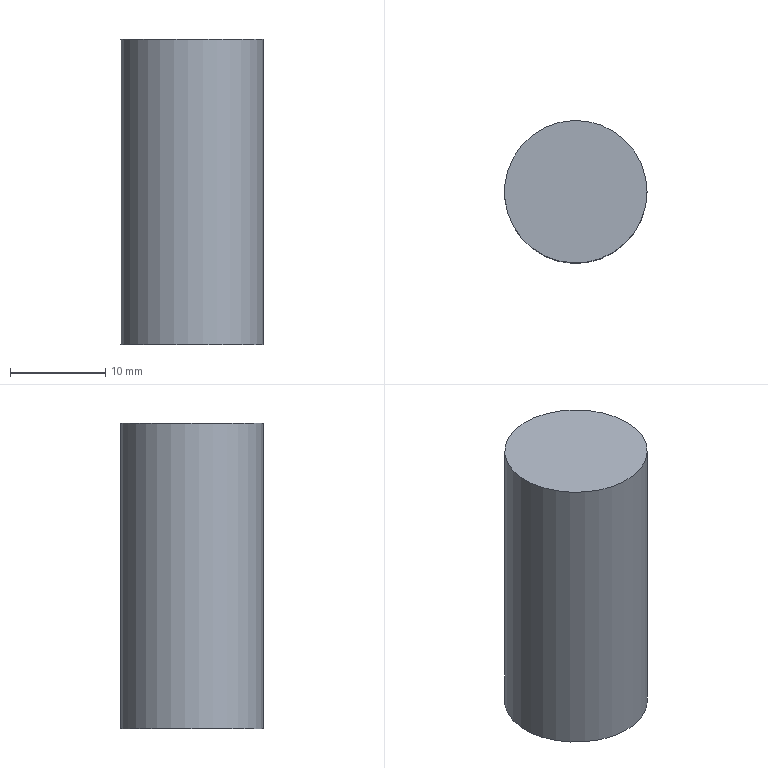Part | NX | features DATUM_CSYS 2, EXTRUDE 1, SKETCH 1 | 1 solid | 3 faces | box 15 x 15 x 32.2 mm | volume 5690 mm3 | plane 2 | cylinder 1 | commonest cylinder face diameters 15 x1
STEP:
#1=CARTESIAN_POINT('',(7.5,0.,32.2));
#2=VERTEX_POINT('',#1);
#3=CARTESIAN_POINT('',(0.,0.,32.2));
#4=DIRECTION('',(0.,0.,1.));
#5=DIRECTION('',(1.,0.,0.));
#6=AXIS2_PLACEMENT_3D('',#3,#4,#5);
#7=CIRCLE('',#6,7.5);
#8=EDGE_CURVE('',#2,#2,#7,.T.);
#9=ORIENTED_EDGE('',*,*,#8,.F.);
#10=EDGE_LOOP('',(#9));
#11=FACE_BOUND('',#10,.T.);
#12=CARTESIAN_POINT('',(7.5,0.,0.));
#13=VERTEX_POINT('',#12);
#14=CARTESIAN_POINT('',(0.,0.,0.));
#15=DIRECTION('',(0.,0.,1.));
#16=DIRECTION('',(1.,0.,0.));
#17=AXIS2_PLACEMENT_3D('',#14,#15,#16);
#18=CIRCLE('',#17,7.5);
#19=EDGE_CURVE('',#13,#13,#18,.T.);
#20=ORIENTED_EDGE('',*,*,#19,.T.);
#21=EDGE_LOOP('',(#20));
#22=FACE_BOUND('',#21,.T.);
#23=CARTESIAN_POINT('',(0.,0.,32.2));
#24=DIRECTION('',(0.,0.,-1.));
#25=DIRECTION('',(-1.,0.,0.));
#26=AXIS2_PLACEMENT_3D('',#23,#24,#25);
#27=CYLINDRICAL_SURFACE('',#26,7.5);
#28=ADVANCED_FACE('',(#11,#22),#27,.T.);
#29=ORIENTED_EDGE('',*,*,#8,.T.);
#30=EDGE_LOOP('',(#29));
#31=FACE_BOUND('',#30,.T.);
#32=CARTESIAN_POINT('',(0.,0.,32.2));
#33=DIRECTION('',(0.,0.,1.));
#34=DIRECTION('',(1.,0.,0.));
#35=AXIS2_PLACEMENT_3D('',#32,#33,#34);
#36=PLANE('',#35);
#37=ADVANCED_FACE('',(#31),#36,.T.);
#38=ORIENTED_EDGE('',*,*,#19,.F.);
#39=EDGE_LOOP('',(#38));
#40=FACE_BOUND('',#39,.T.);
#41=CARTESIAN_POINT('',(0.,0.,0.));
#42=DIRECTION('',(0.,0.,1.));
#43=DIRECTION('',(1.,0.,0.));
#44=AXIS2_PLACEMENT_3D('',#41,#42,#43);
#45=PLANE('',#44);
#46=ADVANCED_FACE('',(#40),#45,.F.);
#47=CLOSED_SHELL('',(#28,#37,#46));
#48=MANIFOLD_SOLID_BREP('',#47);
#49=(LENGTH_UNIT()NAMED_UNIT(*)SI_UNIT(.MILLI.,.METRE.));
#50=UNCERTAINTY_MEASURE_WITH_UNIT(LENGTH_MEASURE(0.00001),#49,'','');
#51=(NAMED_UNIT(*)PLANE_ANGLE_UNIT()SI_UNIT($,.RADIAN.));
#52=(NAMED_UNIT(*)SI_UNIT($,.STERADIAN.)SOLID_ANGLE_UNIT());
#53=(GEOMETRIC_REPRESENTATION_CONTEXT(3)GLOBAL_UNCERTAINTY_ASSIGNED_CONTEXT((#50))GLOBAL_UNIT_ASSIGNED_CONTEXT((#49,#51,#52))REPRESENTATION_CONTEXT('',''));
#54=ADVANCED_BREP_SHAPE_REPRESENTATION('',(#48),#53);